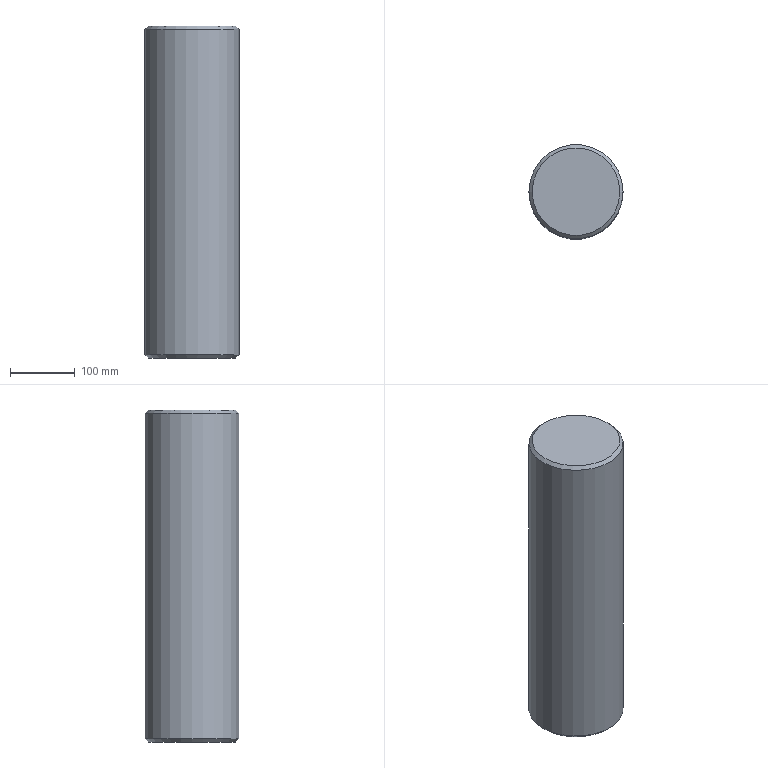Part | NX | features 掩护梁连杆柱销 2 | 1 solid | 5 faces | box 145 x 145 x 511 mm | volume 8427015 mm3 | plane 2 | cone 2 | cylinder 1 | commonest cylinder face diameters 145 x1
STEP:
#1=CARTESIAN_POINT('',(72.5,0.,506.));
#2=VERTEX_POINT('',#1);
#3=CARTESIAN_POINT('',(0.,0.,506.));
#4=DIRECTION('',(0.,0.,1.));
#5=DIRECTION('',(1.,0.,0.));
#6=AXIS2_PLACEMENT_3D('',#3,#4,#5);
#7=CIRCLE('',#6,72.5);
#8=EDGE_CURVE('',#2,#2,#7,.F.);
#9=ORIENTED_EDGE('',*,*,#8,.T.);
#10=EDGE_LOOP('',(#9));
#11=FACE_BOUND('',#10,.T.);
#12=CARTESIAN_POINT('',(72.5,0.,5.));
#13=VERTEX_POINT('',#12);
#14=CARTESIAN_POINT('',(0.,0.,5.));
#15=DIRECTION('',(0.,0.,1.));
#16=DIRECTION('',(1.,0.,0.));
#17=AXIS2_PLACEMENT_3D('',#14,#15,#16);
#18=CIRCLE('',#17,72.5);
#19=EDGE_CURVE('',#13,#13,#18,.T.);
#20=ORIENTED_EDGE('',*,*,#19,.T.);
#21=EDGE_LOOP('',(#20));
#22=FACE_BOUND('',#21,.T.);
#23=CARTESIAN_POINT('',(0.,0.,511.));
#24=DIRECTION('',(0.,0.,-1.));
#25=DIRECTION('',(-1.,0.,0.));
#26=AXIS2_PLACEMENT_3D('',#23,#24,#25);
#27=CYLINDRICAL_SURFACE('',#26,72.5);
#28=ADVANCED_FACE('',(#11,#22),#27,.T.);
#29=CARTESIAN_POINT('',(67.5,0.,511.));
#30=VERTEX_POINT('',#29);
#31=CARTESIAN_POINT('',(0.,0.,511.));
#32=DIRECTION('',(0.,0.,1.));
#33=DIRECTION('',(1.,0.,0.));
#34=AXIS2_PLACEMENT_3D('',#31,#32,#33);
#35=CIRCLE('',#34,67.5);
#36=EDGE_CURVE('',#30,#30,#35,.T.);
#37=ORIENTED_EDGE('',*,*,#36,.T.);
#38=EDGE_LOOP('',(#37));
#39=FACE_BOUND('',#38,.T.);
#40=CARTESIAN_POINT('',(0.,0.,511.));
#41=DIRECTION('',(0.,0.,1.));
#42=DIRECTION('',(1.,0.,0.));
#43=AXIS2_PLACEMENT_3D('',#40,#41,#42);
#44=PLANE('',#43);
#45=ADVANCED_FACE('',(#39),#44,.T.);
#46=CARTESIAN_POINT('',(67.5,0.,0.));
#47=VERTEX_POINT('',#46);
#48=CARTESIAN_POINT('',(0.,0.,0.));
#49=DIRECTION('',(0.,0.,1.));
#50=DIRECTION('',(1.,0.,0.));
#51=AXIS2_PLACEMENT_3D('',#48,#49,#50);
#52=CIRCLE('',#51,67.5);
#53=EDGE_CURVE('',#47,#47,#52,.F.);
#54=ORIENTED_EDGE('',*,*,#53,.T.);
#55=EDGE_LOOP('',(#54));
#56=FACE_BOUND('',#55,.T.);
#57=CARTESIAN_POINT('',(0.,0.,0.));
#58=DIRECTION('',(0.,0.,1.));
#59=DIRECTION('',(1.,0.,0.));
#60=AXIS2_PLACEMENT_3D('',#57,#58,#59);
#61=PLANE('',#60);
#62=ADVANCED_FACE('',(#56),#61,.F.);
#63=ORIENTED_EDGE('',*,*,#8,.F.);
#64=EDGE_LOOP('',(#63));
#65=FACE_BOUND('',#64,.T.);
#66=ORIENTED_EDGE('',*,*,#36,.F.);
#67=EDGE_LOOP('',(#66));
#68=FACE_BOUND('',#67,.T.);
#69=CARTESIAN_POINT('',(0.,0.,511.));
#70=DIRECTION('',(0.,0.,-1.));
#71=DIRECTION('',(-1.,0.,0.));
#72=AXIS2_PLACEMENT_3D('',#69,#70,#71);
#73=CONICAL_SURFACE('',#72,67.5,0.7854);
#74=ADVANCED_FACE('',(#65,#68),#73,.T.);
#75=ORIENTED_EDGE('',*,*,#53,.F.);
#76=EDGE_LOOP('',(#75));
#77=FACE_BOUND('',#76,.T.);
#78=ORIENTED_EDGE('',*,*,#19,.F.);
#79=EDGE_LOOP('',(#78));
#80=FACE_BOUND('',#79,.T.);
#81=CARTESIAN_POINT('',(0.,0.,5.));
#82=DIRECTION('',(0.,0.,1.));
#83=DIRECTION('',(1.,0.,0.));
#84=AXIS2_PLACEMENT_3D('',#81,#82,#83);
#85=CONICAL_SURFACE('',#84,72.5,0.7854);
#86=ADVANCED_FACE('',(#77,#80),#85,.T.);
#87=CLOSED_SHELL('',(#28,#45,#62,#74,#86));
#88=MANIFOLD_SOLID_BREP('',#87);
#89=(LENGTH_UNIT()NAMED_UNIT(*)SI_UNIT(.MILLI.,.METRE.));
#90=UNCERTAINTY_MEASURE_WITH_UNIT(LENGTH_MEASURE(0.00001),#89,'','');
#91=(NAMED_UNIT(*)PLANE_ANGLE_UNIT()SI_UNIT($,.RADIAN.));
#92=(NAMED_UNIT(*)SI_UNIT($,.STERADIAN.)SOLID_ANGLE_UNIT());
#93=(GEOMETRIC_REPRESENTATION_CONTEXT(3)GLOBAL_UNCERTAINTY_ASSIGNED_CONTEXT((#90))GLOBAL_UNIT_ASSIGNED_CONTEXT((#89,#91,#92))REPRESENTATION_CONTEXT('',''));
#94=ADVANCED_BREP_SHAPE_REPRESENTATION('',(#88),#93);